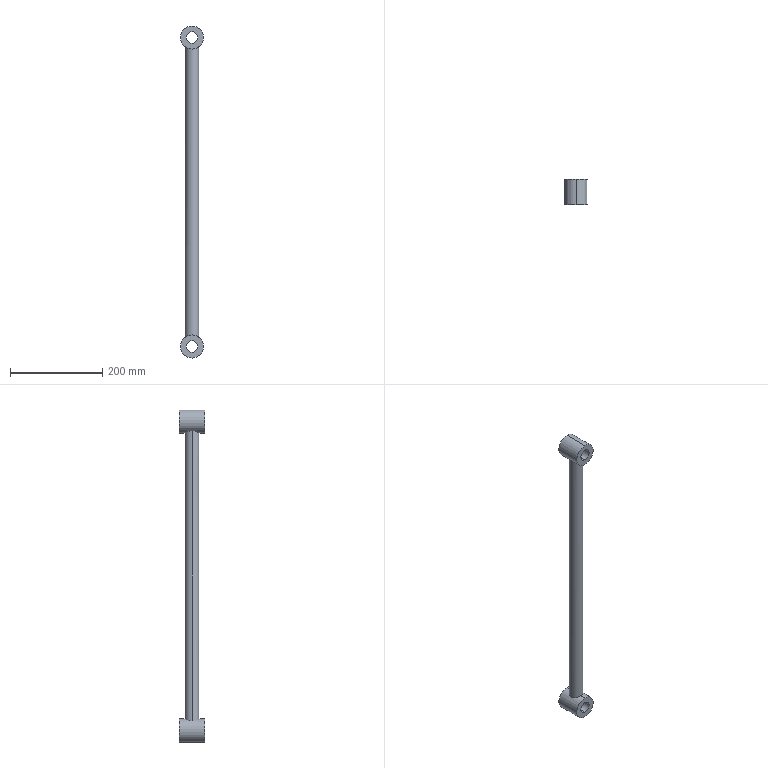Part | STEP file | 1 solid | 19 faces | box 50 x 55 x 720 mm | volume 407064 mm3 | cylinder 15 | plane 4 | commonest cylinder face diameters 50 x7 25 x4 20 x2 30 x2